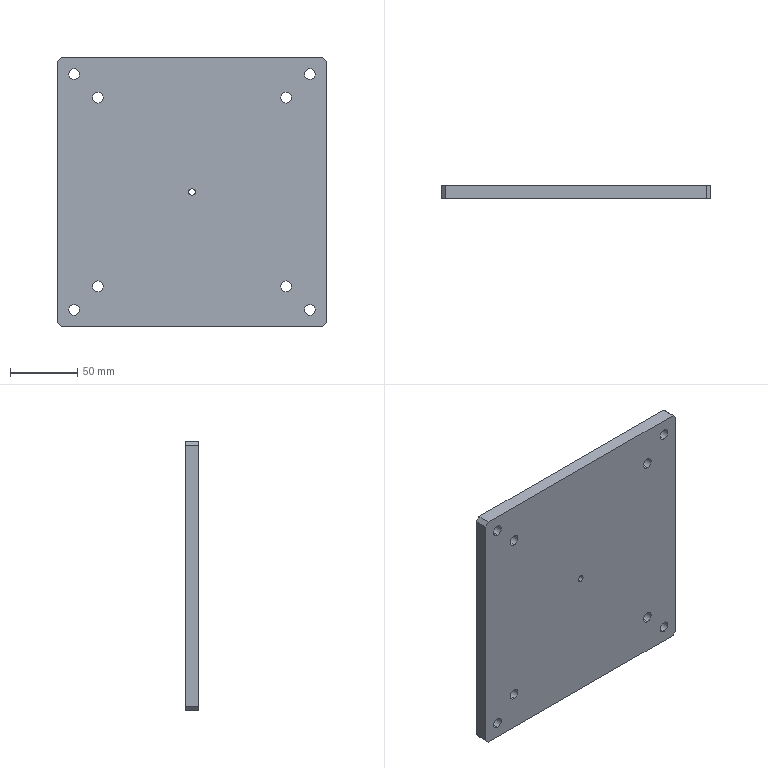Part | STEP file | Guide wheel mechanism revised.sldasm-Part-319 | 1 solid | 28 faces | box 200 x 10 x 200 mm | volume 395602 mm3 | cylinder 18 | plane 10 | commonest cylinder face diameters 8 x16 5 x2
STEP:
#1=CARTESIAN_POINT('',(-70.,10.,66.));
#2=VERTEX_POINT('',#1);
#3=CARTESIAN_POINT('',(-70.,10.,74.));
#4=VERTEX_POINT('',#3);
#5=CARTESIAN_POINT('',(-70.,10.,70.));
#6=DIRECTION('',(0.,1.,0.));
#7=DIRECTION('',(0.,0.,1.));
#8=AXIS2_PLACEMENT_3D('',#5,#6,#7);
#9=CIRCLE('',#8,4.);
#10=EDGE_CURVE('',#2,#4,#9,.T.);
#11=ORIENTED_EDGE('',*,*,#10,.T.);
#12=CARTESIAN_POINT('',(-70.,0.,74.));
#13=VERTEX_POINT('',#12);
#14=CARTESIAN_POINT('',(-70.,10.,74.));
#15=DIRECTION('',(0.,-1.,0.));
#16=VECTOR('',#15,1000.);
#17=LINE('',#14,#16);
#18=EDGE_CURVE('',#4,#13,#17,.T.);
#19=ORIENTED_EDGE('',*,*,#18,.T.);
#20=CARTESIAN_POINT('',(-70.,0.,66.));
#21=VERTEX_POINT('',#20);
#22=CARTESIAN_POINT('',(-70.,0.,70.));
#23=DIRECTION('',(0.,1.,0.));
#24=DIRECTION('',(0.,0.,1.));
#25=AXIS2_PLACEMENT_3D('',#22,#23,#24);
#26=CIRCLE('',#25,4.);
#27=EDGE_CURVE('',#21,#13,#26,.T.);
#28=ORIENTED_EDGE('',*,*,#27,.F.);
#29=CARTESIAN_POINT('',(-70.,10.,66.));
#30=DIRECTION('',(0.,-1.,0.));
#31=VECTOR('',#30,1000.);
#32=LINE('',#29,#31);
#33=EDGE_CURVE('',#2,#21,#32,.T.);
#34=ORIENTED_EDGE('',*,*,#33,.F.);
#35=EDGE_LOOP('',(#11,#19,#28,#34));
#36=FACE_OUTER_BOUND('',#35,.T.);
#37=CARTESIAN_POINT('',(-70.,10.,70.));
#38=DIRECTION('',(0.,-1.,0.));
#39=DIRECTION('',(0.,0.,-1.));
#40=AXIS2_PLACEMENT_3D('',#37,#38,#39);
#41=CYLINDRICAL_SURFACE('',#40,4.);
#42=ADVANCED_FACE('',(#36),#41,.F.);
#43=CARTESIAN_POINT('',(70.,10.,66.));
#44=VERTEX_POINT('',#43);
#45=CARTESIAN_POINT('',(70.,10.,74.));
#46=VERTEX_POINT('',#45);
#47=CARTESIAN_POINT('',(70.,10.,70.));
#48=DIRECTION('',(0.,1.,0.));
#49=DIRECTION('',(0.,0.,1.));
#50=AXIS2_PLACEMENT_3D('',#47,#48,#49);
#51=CIRCLE('',#50,4.);
#52=EDGE_CURVE('',#44,#46,#51,.T.);
#53=ORIENTED_EDGE('',*,*,#52,.T.);
#54=CARTESIAN_POINT('',(70.,0.,74.));
#55=VERTEX_POINT('',#54);
#56=CARTESIAN_POINT('',(70.,10.,74.));
#57=DIRECTION('',(0.,-1.,0.));
#58=VECTOR('',#57,1000.);
#59=LINE('',#56,#58);
#60=EDGE_CURVE('',#46,#55,#59,.T.);
#61=ORIENTED_EDGE('',*,*,#60,.T.);
#62=CARTESIAN_POINT('',(70.,0.,66.));
#63=VERTEX_POINT('',#62);
#64=CARTESIAN_POINT('',(70.,0.,70.));
#65=DIRECTION('',(0.,1.,0.));
#66=DIRECTION('',(0.,0.,1.));
#67=AXIS2_PLACEMENT_3D('',#64,#65,#66);
#68=CIRCLE('',#67,4.);
#69=EDGE_CURVE('',#63,#55,#68,.T.);
#70=ORIENTED_EDGE('',*,*,#69,.F.);
#71=CARTESIAN_POINT('',(70.,10.,66.));
#72=DIRECTION('',(0.,-1.,0.));
#73=VECTOR('',#72,1000.);
#74=LINE('',#71,#73);
#75=EDGE_CURVE('',#44,#63,#74,.T.);
#76=ORIENTED_EDGE('',*,*,#75,.F.);
#77=EDGE_LOOP('',(#53,#61,#70,#76));
#78=FACE_OUTER_BOUND('',#77,.T.);
#79=CARTESIAN_POINT('',(70.,10.,70.));
#80=DIRECTION('',(0.,-1.,0.));
#81=DIRECTION('',(0.,0.,-1.));
#82=AXIS2_PLACEMENT_3D('',#79,#80,#81);
#83=CYLINDRICAL_SURFACE('',#82,4.);
#84=ADVANCED_FACE('',(#78),#83,.F.);
#85=CARTESIAN_POINT('',(70.,10.,-74.));
#86=VERTEX_POINT('',#85);
#87=CARTESIAN_POINT('',(70.,10.,-66.));
#88=VERTEX_POINT('',#87);
#89=CARTESIAN_POINT('',(70.,10.,-70.));
#90=DIRECTION('',(0.,1.,0.));
#91=DIRECTION('',(0.,0.,1.));
#92=AXIS2_PLACEMENT_3D('',#89,#90,#91);
#93=CIRCLE('',#92,4.);
#94=EDGE_CURVE('',#86,#88,#93,.T.);
#95=ORIENTED_EDGE('',*,*,#94,.T.);
#96=CARTESIAN_POINT('',(70.,0.,-66.));
#97=VERTEX_POINT('',#96);
#98=CARTESIAN_POINT('',(70.,10.,-66.));
#99=DIRECTION('',(0.,-1.,0.));
#100=VECTOR('',#99,1000.);
#101=LINE('',#98,#100);
#102=EDGE_CURVE('',#88,#97,#101,.T.);
#103=ORIENTED_EDGE('',*,*,#102,.T.);
#104=CARTESIAN_POINT('',(70.,0.,-74.));
#105=VERTEX_POINT('',#104);
#106=CARTESIAN_POINT('',(70.,0.,-70.));
#107=DIRECTION('',(0.,1.,0.));
#108=DIRECTION('',(0.,0.,1.));
#109=AXIS2_PLACEMENT_3D('',#106,#107,#108);
#110=CIRCLE('',#109,4.);
#111=EDGE_CURVE('',#105,#97,#110,.T.);
#112=ORIENTED_EDGE('',*,*,#111,.F.);
#113=CARTESIAN_POINT('',(70.,10.,-74.));
#114=DIRECTION('',(0.,-1.,0.));
#115=VECTOR('',#114,1000.);
#116=LINE('',#113,#115);
#117=EDGE_CURVE('',#86,#105,#116,.T.);
#118=ORIENTED_EDGE('',*,*,#117,.F.);
#119=EDGE_LOOP('',(#95,#103,#112,#118));
#120=FACE_OUTER_BOUND('',#119,.T.);
#121=CARTESIAN_POINT('',(70.,10.,-70.));
#122=DIRECTION('',(0.,-1.,0.));
#123=DIRECTION('',(0.,0.,-1.));
#124=AXIS2_PLACEMENT_3D('',#121,#122,#123);
#125=CYLINDRICAL_SURFACE('',#124,4.);
#126=ADVANCED_FACE('',(#120),#125,.F.);
#127=CARTESIAN_POINT('',(-70.,10.,-74.));
#128=VERTEX_POINT('',#127);
#129=CARTESIAN_POINT('',(-70.,10.,-66.));
#130=VERTEX_POINT('',#129);
#131=CARTESIAN_POINT('',(-70.,10.,-70.));
#132=DIRECTION('',(0.,1.,0.));
#133=DIRECTION('',(0.,0.,1.));
#134=AXIS2_PLACEMENT_3D('',#131,#132,#133);
#135=CIRCLE('',#134,4.);
#136=EDGE_CURVE('',#128,#130,#135,.T.);
#137=ORIENTED_EDGE('',*,*,#136,.T.);
#138=CARTESIAN_POINT('',(-70.,0.,-66.));
#139=VERTEX_POINT('',#138);
#140=CARTESIAN_POINT('',(-70.,10.,-66.));
#141=DIRECTION('',(0.,-1.,0.));
#142=VECTOR('',#141,1000.);
#143=LINE('',#140,#142);
#144=EDGE_CURVE('',#130,#139,#143,.T.);
#145=ORIENTED_EDGE('',*,*,#144,.T.);
#146=CARTESIAN_POINT('',(-70.,0.,-74.));
#147=VERTEX_POINT('',#146);
#148=CARTESIAN_POINT('',(-70.,0.,-70.));
#149=DIRECTION('',(0.,1.,0.));
#150=DIRECTION('',(0.,0.,1.));
#151=AXIS2_PLACEMENT_3D('',#148,#149,#150);
#152=CIRCLE('',#151,4.);
#153=EDGE_CURVE('',#147,#139,#152,.T.);
#154=ORIENTED_EDGE('',*,*,#153,.F.);
#155=CARTESIAN_POINT('',(-70.,10.,-74.));
#156=DIRECTION('',(0.,-1.,0.));
#157=VECTOR('',#156,1000.);
#158=LINE('',#155,#157);
#159=EDGE_CURVE('',#128,#147,#158,.T.);
#160=ORIENTED_EDGE('',*,*,#159,.F.);
#161=EDGE_LOOP('',(#137,#145,#154,#160));
#162=FACE_OUTER_BOUND('',#161,.T.);
#163=CARTESIAN_POINT('',(-70.,10.,-70.));
#164=DIRECTION('',(0.,-1.,0.));
#165=DIRECTION('',(0.,0.,-1.));
#166=AXIS2_PLACEMENT_3D('',#163,#164,#165);
#167=CYLINDRICAL_SURFACE('',#166,4.);
#168=ADVANCED_FACE('',(#162),#167,.F.);
#169=CARTESIAN_POINT('',(-87.5,10.,83.5));
#170=VERTEX_POINT('',#169);
#171=CARTESIAN_POINT('',(-87.5,10.,91.5));
#172=VERTEX_POINT('',#171);
#173=CARTESIAN_POINT('',(-87.5,10.,87.5));
#174=DIRECTION('',(0.,1.,0.));
#175=DIRECTION('',(0.,0.,1.));
#176=AXIS2_PLACEMENT_3D('',#173,#174,#175);
#177=CIRCLE('',#176,4.);
#178=EDGE_CURVE('',#170,#172,#177,.T.);
#179=ORIENTED_EDGE('',*,*,#178,.T.);
#180=CARTESIAN_POINT('',(-87.5,0.,91.5));
#181=VERTEX_POINT('',#180);
#182=CARTESIAN_POINT('',(-87.5,10.,91.5));
#183=DIRECTION('',(0.,-1.,0.));
#184=VECTOR('',#183,1000.);
#185=LINE('',#182,#184);
#186=EDGE_CURVE('',#172,#181,#185,.T.);
#187=ORIENTED_EDGE('',*,*,#186,.T.);
#188=CARTESIAN_POINT('',(-87.5,0.,83.5));
#189=VERTEX_POINT('',#188);
#190=CARTESIAN_POINT('',(-87.5,0.,87.5));
#191=DIRECTION('',(0.,1.,0.));
#192=DIRECTION('',(0.,0.,1.));
#193=AXIS2_PLACEMENT_3D('',#190,#191,#192);
#194=CIRCLE('',#193,4.);
#195=EDGE_CURVE('',#189,#181,#194,.T.);
#196=ORIENTED_EDGE('',*,*,#195,.F.);
#197=CARTESIAN_POINT('',(-87.5,10.,83.5));
#198=DIRECTION('',(0.,-1.,0.));
#199=VECTOR('',#198,1000.);
#200=LINE('',#197,#199);
#201=EDGE_CURVE('',#170,#189,#200,.T.);
#202=ORIENTED_EDGE('',*,*,#201,.F.);
#203=EDGE_LOOP('',(#179,#187,#196,#202));
#204=FACE_OUTER_BOUND('',#203,.T.);
#205=CARTESIAN_POINT('',(-87.5,10.,87.5));
#206=DIRECTION('',(0.,-1.,0.));
#207=DIRECTION('',(0.,0.,-1.));
#208=AXIS2_PLACEMENT_3D('',#205,#206,#207);
#209=CYLINDRICAL_SURFACE('',#208,4.);
#210=ADVANCED_FACE('',(#204),#209,.F.);
#211=CARTESIAN_POINT('',(87.5,10.,83.5));
#212=VERTEX_POINT('',#211);
#213=CARTESIAN_POINT('',(87.5,10.,91.5));
#214=VERTEX_POINT('',#213);
#215=CARTESIAN_POINT('',(87.5,10.,87.5));
#216=DIRECTION('',(0.,1.,0.));
#217=DIRECTION('',(0.,0.,1.));
#218=AXIS2_PLACEMENT_3D('',#215,#216,#217);
#219=CIRCLE('',#218,4.);
#220=EDGE_CURVE('',#212,#214,#219,.T.);
#221=ORIENTED_EDGE('',*,*,#220,.T.);
#222=CARTESIAN_POINT('',(87.5,0.,91.5));
#223=VERTEX_POINT('',#222);
#224=CARTESIAN_POINT('',(87.5,10.,91.5));
#225=DIRECTION('',(0.,-1.,0.));
#226=VECTOR('',#225,1000.);
#227=LINE('',#224,#226);
#228=EDGE_CURVE('',#214,#223,#227,.T.);
#229=ORIENTED_EDGE('',*,*,#228,.T.);
#230=CARTESIAN_POINT('',(87.5,0.,83.5));
#231=VERTEX_POINT('',#230);
#232=CARTESIAN_POINT('',(87.5,0.,87.5));
#233=DIRECTION('',(0.,1.,0.));
#234=DIRECTION('',(0.,0.,1.));
#235=AXIS2_PLACEMENT_3D('',#232,#233,#234);
#236=CIRCLE('',#235,4.);
#237=EDGE_CURVE('',#231,#223,#236,.T.);
#238=ORIENTED_EDGE('',*,*,#237,.F.);
#239=CARTESIAN_POINT('',(87.5,10.,83.5));
#240=DIRECTION('',(0.,-1.,0.));
#241=VECTOR('',#240,1000.);
#242=LINE('',#239,#241);
#243=EDGE_CURVE('',#212,#231,#242,.T.);
#244=ORIENTED_EDGE('',*,*,#243,.F.);
#245=EDGE_LOOP('',(#221,#229,#238,#244));
#246=FACE_OUTER_BOUND('',#245,.T.);
#247=CARTESIAN_POINT('',(87.5,10.,87.5));
#248=DIRECTION('',(0.,-1.,0.));
#249=DIRECTION('',(0.,0.,-1.));
#250=AXIS2_PLACEMENT_3D('',#247,#248,#249);
#251=CYLINDRICAL_SURFACE('',#250,4.);
#252=ADVANCED_FACE('',(#246),#251,.F.);
#253=CARTESIAN_POINT('',(87.5,10.,-91.5));
#254=VERTEX_POINT('',#253);
#255=CARTESIAN_POINT('',(87.5,10.,-83.5));
#256=VERTEX_POINT('',#255);
#257=CARTESIAN_POINT('',(87.5,10.,-87.5));
#258=DIRECTION('',(0.,1.,0.));
#259=DIRECTION('',(0.,0.,1.));
#260=AXIS2_PLACEMENT_3D('',#257,#258,#259);
#261=CIRCLE('',#260,4.);
#262=EDGE_CURVE('',#254,#256,#261,.T.);
#263=ORIENTED_EDGE('',*,*,#262,.T.);
#264=CARTESIAN_POINT('',(87.5,0.,-83.5));
#265=VERTEX_POINT('',#264);
#266=CARTESIAN_POINT('',(87.5,10.,-83.5));
#267=DIRECTION('',(0.,-1.,0.));
#268=VECTOR('',#267,1000.);
#269=LINE('',#266,#268);
#270=EDGE_CURVE('',#256,#265,#269,.T.);
#271=ORIENTED_EDGE('',*,*,#270,.T.);
#272=CARTESIAN_POINT('',(87.5,0.,-91.5));
#273=VERTEX_POINT('',#272);
#274=CARTESIAN_POINT('',(87.5,0.,-87.5));
#275=DIRECTION('',(0.,1.,0.));
#276=DIRECTION('',(0.,0.,1.));
#277=AXIS2_PLACEMENT_3D('',#274,#275,#276);
#278=CIRCLE('',#277,4.);
#279=EDGE_CURVE('',#273,#265,#278,.T.);
#280=ORIENTED_EDGE('',*,*,#279,.F.);
#281=CARTESIAN_POINT('',(87.5,10.,-91.5));
#282=DIRECTION('',(0.,-1.,0.));
#283=VECTOR('',#282,1000.);
#284=LINE('',#281,#283);
#285=EDGE_CURVE('',#254,#273,#284,.T.);
#286=ORIENTED_EDGE('',*,*,#285,.F.);
#287=EDGE_LOOP('',(#263,#271,#280,#286));
#288=FACE_OUTER_BOUND('',#287,.T.);
#289=CARTESIAN_POINT('',(87.5,10.,-87.5));
#290=DIRECTION('',(0.,-1.,0.));
#291=DIRECTION('',(0.,0.,-1.));
#292=AXIS2_PLACEMENT_3D('',#289,#290,#291);
#293=CYLINDRICAL_SURFACE('',#292,4.);
#294=ADVANCED_FACE('',(#288),#293,.F.);
#295=CARTESIAN_POINT('',(-87.5,10.,-91.5));
#296=VERTEX_POINT('',#295);
#297=CARTESIAN_POINT('',(-87.5,10.,-83.5));
#298=VERTEX_POINT('',#297);
#299=CARTESIAN_POINT('',(-87.5,10.,-87.5));
#300=DIRECTION('',(0.,1.,0.));
#301=DIRECTION('',(0.,0.,1.));
#302=AXIS2_PLACEMENT_3D('',#299,#300,#301);
#303=CIRCLE('',#302,4.);
#304=EDGE_CURVE('',#296,#298,#303,.T.);
#305=ORIENTED_EDGE('',*,*,#304,.T.);
#306=CARTESIAN_POINT('',(-87.5,0.,-83.5));
#307=VERTEX_POINT('',#306);
#308=CARTESIAN_POINT('',(-87.5,10.,-83.5));
#309=DIRECTION('',(0.,-1.,0.));
#310=VECTOR('',#309,1000.);
#311=LINE('',#308,#310);
#312=EDGE_CURVE('',#298,#307,#311,.T.);
#313=ORIENTED_EDGE('',*,*,#312,.T.);
#314=CARTESIAN_POINT('',(-87.5,0.,-91.5));
#315=VERTEX_POINT('',#314);
#316=CARTESIAN_POINT('',(-87.5,0.,-87.5));
#317=DIRECTION('',(0.,1.,0.));
#318=DIRECTION('',(0.,0.,1.));
#319=AXIS2_PLACEMENT_3D('',#316,#317,#318);
#320=CIRCLE('',#319,4.);
#321=EDGE_CURVE('',#315,#307,#320,.T.);
#322=ORIENTED_EDGE('',*,*,#321,.F.);
#323=CARTESIAN_POINT('',(-87.5,10.,-91.5));
#324=DIRECTION('',(0.,-1.,0.));
#325=VECTOR('',#324,1000.);
#326=LINE('',#323,#325);
#327=EDGE_CURVE('',#296,#315,#326,.T.);
#328=ORIENTED_EDGE('',*,*,#327,.F.);
#329=EDGE_LOOP('',(#305,#313,#322,#328));
#330=FACE_OUTER_BOUND('',#329,.T.);
#331=CARTESIAN_POINT('',(-87.5,10.,-87.5));
#332=DIRECTION('',(0.,-1.,0.));
#333=DIRECTION('',(0.,0.,-1.));
#334=AXIS2_PLACEMENT_3D('',#331,#332,#333);
#335=CYLINDRICAL_SURFACE('',#334,4.);
#336=ADVANCED_FACE('',(#330),#335,.F.);
#337=CARTESIAN_POINT('',(0.,10.,-2.5));
#338=VERTEX_POINT('',#337);
#339=CARTESIAN_POINT('',(0.,10.,2.5));
#340=VERTEX_POINT('',#339);
#341=CARTESIAN_POINT('',(0.,10.,0.));
#342=DIRECTION('',(0.,1.,0.));
#343=DIRECTION('',(0.,0.,1.));
#344=AXIS2_PLACEMENT_3D('',#341,#342,#343);
#345=CIRCLE('',#344,2.5);
#346=EDGE_CURVE('',#338,#340,#345,.T.);
#347=ORIENTED_EDGE('',*,*,#346,.T.);
#348=CARTESIAN_POINT('',(0.,0.,2.5));
#349=VERTEX_POINT('',#348);
#350=CARTESIAN_POINT('',(0.,10.,2.5));
#351=DIRECTION('',(0.,-1.,0.));
#352=VECTOR('',#351,1000.);
#353=LINE('',#350,#352);
#354=EDGE_CURVE('',#340,#349,#353,.T.);
#355=ORIENTED_EDGE('',*,*,#354,.T.);
#356=CARTESIAN_POINT('',(0.,0.,-2.5));
#357=VERTEX_POINT('',#356);
#358=CARTESIAN_POINT('',(0.,0.,0.));
#359=DIRECTION('',(0.,1.,0.));
#360=DIRECTION('',(0.,0.,1.));
#361=AXIS2_PLACEMENT_3D('',#358,#359,#360);
#362=CIRCLE('',#361,2.5);
#363=EDGE_CURVE('',#357,#349,#362,.T.);
#364=ORIENTED_EDGE('',*,*,#363,.F.);
#365=CARTESIAN_POINT('',(0.,10.,-2.5));
#366=DIRECTION('',(0.,-1.,0.));
#367=VECTOR('',#366,1000.);
#368=LINE('',#365,#367);
#369=EDGE_CURVE('',#338,#357,#368,.T.);
#370=ORIENTED_EDGE('',*,*,#369,.F.);
#371=EDGE_LOOP('',(#347,#355,#364,#370));
#372=FACE_OUTER_BOUND('',#371,.T.);
#373=CARTESIAN_POINT('',(0.,10.,0.));
#374=DIRECTION('',(0.,-1.,0.));
#375=DIRECTION('',(0.,0.,-1.));
#376=AXIS2_PLACEMENT_3D('',#373,#374,#375);
#377=CYLINDRICAL_SURFACE('',#376,2.5);
#378=ADVANCED_FACE('',(#372),#377,.F.);
#379=ORIENTED_EDGE('',*,*,#52,.F.);
#380=CARTESIAN_POINT('',(70.,10.,70.));
#381=DIRECTION('',(0.,1.,0.));
#382=DIRECTION('',(0.,0.,1.));
#383=AXIS2_PLACEMENT_3D('',#380,#381,#382);
#384=CIRCLE('',#383,4.);
#385=EDGE_CURVE('',#46,#44,#384,.T.);
#386=ORIENTED_EDGE('',*,*,#385,.F.);
#387=EDGE_LOOP('',(#379,#386));
#388=FACE_BOUND('',#387,.T.);
#389=ORIENTED_EDGE('',*,*,#136,.F.);
#390=CARTESIAN_POINT('',(-70.,10.,-70.));
#391=DIRECTION('',(0.,1.,0.));
#392=DIRECTION('',(0.,0.,1.));
#393=AXIS2_PLACEMENT_3D('',#390,#391,#392);
#394=CIRCLE('',#393,4.);
#395=EDGE_CURVE('',#130,#128,#394,.T.);
#396=ORIENTED_EDGE('',*,*,#395,.F.);
#397=EDGE_LOOP('',(#389,#396));
#398=FACE_BOUND('',#397,.T.);
#399=ORIENTED_EDGE('',*,*,#220,.F.);
#400=CARTESIAN_POINT('',(87.5,10.,87.5));
#401=DIRECTION('',(0.,1.,0.));
#402=DIRECTION('',(0.,0.,1.));
#403=AXIS2_PLACEMENT_3D('',#400,#401,#402);
#404=CIRCLE('',#403,4.);
#405=EDGE_CURVE('',#214,#212,#404,.T.);
#406=ORIENTED_EDGE('',*,*,#405,.F.);
#407=EDGE_LOOP('',(#399,#406));
#408=FACE_BOUND('',#407,.T.);
#409=ORIENTED_EDGE('',*,*,#304,.F.);
#410=CARTESIAN_POINT('',(-87.5,10.,-87.5));
#411=DIRECTION('',(0.,1.,0.));
#412=DIRECTION('',(0.,0.,1.));
#413=AXIS2_PLACEMENT_3D('',#410,#411,#412);
#414=CIRCLE('',#413,4.);
#415=EDGE_CURVE('',#298,#296,#414,.T.);
#416=ORIENTED_EDGE('',*,*,#415,.F.);
#417=EDGE_LOOP('',(#409,#416));
#418=FACE_BOUND('',#417,.T.);
#419=CARTESIAN_POINT('',(-100.,10.,-97.));
#420=VERTEX_POINT('',#419);
#421=CARTESIAN_POINT('',(-100.,10.,97.));
#422=VERTEX_POINT('',#421);
#423=CARTESIAN_POINT('',(-100.,10.,100.));
#424=DIRECTION('',(0.,0.,1.));
#425=VECTOR('',#424,1000.);
#426=LINE('',#423,#425);
#427=EDGE_CURVE('',#420,#422,#426,.T.);
#428=ORIENTED_EDGE('',*,*,#427,.T.);
#429=CARTESIAN_POINT('',(-97.,10.,100.));
#430=VERTEX_POINT('',#429);
#431=CARTESIAN_POINT('',(-98.5,10.,98.5));
#432=DIRECTION('',(0.7071,0.,0.7071));
#433=VECTOR('',#432,1000.);
#434=LINE('',#431,#433);
#435=EDGE_CURVE('',#422,#430,#434,.T.);
#436=ORIENTED_EDGE('',*,*,#435,.T.);
#437=CARTESIAN_POINT('',(97.,10.,100.));
#438=VERTEX_POINT('',#437);
#439=CARTESIAN_POINT('',(100.,10.,100.));
#440=DIRECTION('',(1.,0.,0.));
#441=VECTOR('',#440,1000.);
#442=LINE('',#439,#441);
#443=EDGE_CURVE('',#430,#438,#442,.T.);
#444=ORIENTED_EDGE('',*,*,#443,.T.);
#445=CARTESIAN_POINT('',(100.,10.,97.));
#446=VERTEX_POINT('',#445);
#447=CARTESIAN_POINT('',(98.5,10.,98.5));
#448=DIRECTION('',(0.7071,0.,-0.7071));
#449=VECTOR('',#448,1000.);
#450=LINE('',#447,#449);
#451=EDGE_CURVE('',#438,#446,#450,.T.);
#452=ORIENTED_EDGE('',*,*,#451,.T.);
#453=CARTESIAN_POINT('',(100.,10.,-97.));
#454=VERTEX_POINT('',#453);
#455=CARTESIAN_POINT('',(100.,10.,100.));
#456=DIRECTION('',(0.,0.,-1.));
#457=VECTOR('',#456,1000.);
#458=LINE('',#455,#457);
#459=EDGE_CURVE('',#446,#454,#458,.T.);
#460=ORIENTED_EDGE('',*,*,#459,.T.);
#461=CARTESIAN_POINT('',(97.,10.,-100.));
#462=VERTEX_POINT('',#461);
#463=CARTESIAN_POINT('',(98.5,10.,-98.5));
#464=DIRECTION('',(-0.7071,0.,-0.7071));
#465=VECTOR('',#464,1000.);
#466=LINE('',#463,#465);
#467=EDGE_CURVE('',#454,#462,#466,.T.);
#468=ORIENTED_EDGE('',*,*,#467,.T.);
#469=CARTESIAN_POINT('',(-97.,10.,-100.));
#470=VERTEX_POINT('',#469);
#471=CARTESIAN_POINT('',(100.,10.,-100.));
#472=DIRECTION('',(-1.,0.,0.));
#473=VECTOR('',#472,1000.);
#474=LINE('',#471,#473);
#475=EDGE_CURVE('',#462,#470,#474,.T.);
#476=ORIENTED_EDGE('',*,*,#475,.T.);
#477=CARTESIAN_POINT('',(-98.5,10.,-98.5));
#478=DIRECTION('',(-0.7071,0.,0.7071));
#479=VECTOR('',#478,1000.);
#480=LINE('',#477,#479);
#481=EDGE_CURVE('',#470,#420,#480,.T.);
#482=ORIENTED_EDGE('',*,*,#481,.T.);
#483=EDGE_LOOP('',(#428,#436,#444,#452,#460,#468,#476,#482));
#484=FACE_OUTER_BOUND('',#483,.T.);
#485=ORIENTED_EDGE('',*,*,#346,.F.);
#486=CARTESIAN_POINT('',(0.,10.,0.));
#487=DIRECTION('',(0.,1.,0.));
#488=DIRECTION('',(0.,0.,1.));
#489=AXIS2_PLACEMENT_3D('',#486,#487,#488);
#490=CIRCLE('',#489,2.5);
#491=EDGE_CURVE('',#340,#338,#490,.T.);
#492=ORIENTED_EDGE('',*,*,#491,.F.);
#493=EDGE_LOOP('',(#485,#492));
#494=FACE_BOUND('',#493,.T.);
#495=ORIENTED_EDGE('',*,*,#262,.F.);
#496=CARTESIAN_POINT('',(87.5,10.,-87.5));
#497=DIRECTION('',(0.,1.,0.));
#498=DIRECTION('',(0.,0.,1.));
#499=AXIS2_PLACEMENT_3D('',#496,#497,#498);
#500=CIRCLE('',#499,4.);
#501=EDGE_CURVE('',#256,#254,#500,.T.);
#502=ORIENTED_EDGE('',*,*,#501,.F.);
#503=EDGE_LOOP('',(#495,#502));
#504=FACE_BOUND('',#503,.T.);
#505=ORIENTED_EDGE('',*,*,#178,.F.);
#506=CARTESIAN_POINT('',(-87.5,10.,87.5));
#507=DIRECTION('',(0.,1.,0.));
#508=DIRECTION('',(0.,0.,1.));
#509=AXIS2_PLACEMENT_3D('',#506,#507,#508);
#510=CIRCLE('',#509,4.);
#511=EDGE_CURVE('',#172,#170,#510,.T.);
#512=ORIENTED_EDGE('',*,*,#511,.F.);
#513=EDGE_LOOP('',(#505,#512));
#514=FACE_BOUND('',#513,.T.);
#515=ORIENTED_EDGE('',*,*,#94,.F.);
#516=CARTESIAN_POINT('',(70.,10.,-70.));
#517=DIRECTION('',(0.,1.,0.));
#518=DIRECTION('',(0.,0.,1.));
#519=AXIS2_PLACEMENT_3D('',#516,#517,#518);
#520=CIRCLE('',#519,4.);
#521=EDGE_CURVE('',#88,#86,#520,.T.);
#522=ORIENTED_EDGE('',*,*,#521,.F.);
#523=EDGE_LOOP('',(#515,#522));
#524=FACE_BOUND('',#523,.T.);
#525=ORIENTED_EDGE('',*,*,#10,.F.);
#526=CARTESIAN_POINT('',(-70.,10.,70.));
#527=DIRECTION('',(0.,1.,0.));
#528=DIRECTION('',(0.,0.,1.));
#529=AXIS2_PLACEMENT_3D('',#526,#527,#528);
#530=CIRCLE('',#529,4.);
#531=EDGE_CURVE('',#4,#2,#530,.T.);
#532=ORIENTED_EDGE('',*,*,#531,.F.);
#533=EDGE_LOOP('',(#525,#532));
#534=FACE_BOUND('',#533,.T.);
#535=CARTESIAN_POINT('',(0.,10.,0.));
#536=DIRECTION('',(0.,1.,0.));
#537=DIRECTION('',(0.,0.,1.));
#538=AXIS2_PLACEMENT_3D('',#535,#536,#537);
#539=PLANE('',#538);
#540=ADVANCED_FACE('',(#388,#398,#408,#418,#484,#494,#504,#514,#524,#534),#539,.T.);
#541=ORIENTED_EDGE('',*,*,#69,.T.);
#542=CARTESIAN_POINT('',(70.,0.,70.));
#543=DIRECTION('',(0.,1.,0.));
#544=DIRECTION('',(0.,0.,1.));
#545=AXIS2_PLACEMENT_3D('',#542,#543,#544);
#546=CIRCLE('',#545,4.);
#547=EDGE_CURVE('',#55,#63,#546,.T.);
#548=ORIENTED_EDGE('',*,*,#547,.T.);
#549=EDGE_LOOP('',(#541,#548));
#550=FACE_BOUND('',#549,.T.);
#551=ORIENTED_EDGE('',*,*,#153,.T.);
#552=CARTESIAN_POINT('',(-70.,0.,-70.));
#553=DIRECTION('',(0.,1.,0.));
#554=DIRECTION('',(0.,0.,1.));
#555=AXIS2_PLACEMENT_3D('',#552,#553,#554);
#556=CIRCLE('',#555,4.);
#557=EDGE_CURVE('',#139,#147,#556,.T.);
#558=ORIENTED_EDGE('',*,*,#557,.T.);
#559=EDGE_LOOP('',(#551,#558));
#560=FACE_BOUND('',#559,.T.);
#561=ORIENTED_EDGE('',*,*,#237,.T.);
#562=CARTESIAN_POINT('',(87.5,0.,87.5));
#563=DIRECTION('',(0.,1.,0.));
#564=DIRECTION('',(0.,0.,1.));
#565=AXIS2_PLACEMENT_3D('',#562,#563,#564);
#566=CIRCLE('',#565,4.);
#567=EDGE_CURVE('',#223,#231,#566,.T.);
#568=ORIENTED_EDGE('',*,*,#567,.T.);
#569=EDGE_LOOP('',(#561,#568));
#570=FACE_BOUND('',#569,.T.);
#571=ORIENTED_EDGE('',*,*,#321,.T.);
#572=CARTESIAN_POINT('',(-87.5,0.,-87.5));
#573=DIRECTION('',(0.,1.,0.));
#574=DIRECTION('',(0.,0.,1.));
#575=AXIS2_PLACEMENT_3D('',#572,#573,#574);
#576=CIRCLE('',#575,4.);
#577=EDGE_CURVE('',#307,#315,#576,.T.);
#578=ORIENTED_EDGE('',*,*,#577,.T.);
#579=EDGE_LOOP('',(#571,#578));
#580=FACE_BOUND('',#579,.T.);
#581=CARTESIAN_POINT('',(-97.,0.,100.));
#582=VERTEX_POINT('',#581);
#583=CARTESIAN_POINT('',(97.,0.,100.));
#584=VERTEX_POINT('',#583);
#585=CARTESIAN_POINT('',(100.,0.,100.));
#586=DIRECTION('',(1.,0.,0.));
#587=VECTOR('',#586,1000.);
#588=LINE('',#585,#587);
#589=EDGE_CURVE('',#582,#584,#588,.T.);
#590=ORIENTED_EDGE('',*,*,#589,.F.);
#591=CARTESIAN_POINT('',(-100.,0.,97.));
#592=VERTEX_POINT('',#591);
#593=CARTESIAN_POINT('',(-97.,0.,100.));
#594=DIRECTION('',(-0.7071,0.,-0.7071));
#595=VECTOR('',#594,1000.);
#596=LINE('',#593,#595);
#597=EDGE_CURVE('',#582,#592,#596,.T.);
#598=ORIENTED_EDGE('',*,*,#597,.T.);
#599=CARTESIAN_POINT('',(-100.,0.,-97.));
#600=VERTEX_POINT('',#599);
#601=CARTESIAN_POINT('',(-100.,0.,100.));
#602=DIRECTION('',(0.,0.,1.));
#603=VECTOR('',#602,1000.);
#604=LINE('',#601,#603);
#605=EDGE_CURVE('',#600,#592,#604,.T.);
#606=ORIENTED_EDGE('',*,*,#605,.F.);
#607=CARTESIAN_POINT('',(-97.,0.,-100.));
#608=VERTEX_POINT('',#607);
#609=CARTESIAN_POINT('',(-100.,0.,-97.));
#610=DIRECTION('',(0.7071,0.,-0.7071));
#611=VECTOR('',#610,1000.);
#612=LINE('',#609,#611);
#613=EDGE_CURVE('',#600,#608,#612,.T.);
#614=ORIENTED_EDGE('',*,*,#613,.T.);
#615=CARTESIAN_POINT('',(97.,0.,-100.));
#616=VERTEX_POINT('',#615);
#617=CARTESIAN_POINT('',(100.,0.,-100.));
#618=DIRECTION('',(-1.,0.,0.));
#619=VECTOR('',#618,1000.);
#620=LINE('',#617,#619);
#621=EDGE_CURVE('',#616,#608,#620,.T.);
#622=ORIENTED_EDGE('',*,*,#621,.F.);
#623=CARTESIAN_POINT('',(100.,0.,-97.));
#624=VERTEX_POINT('',#623);
#625=CARTESIAN_POINT('',(97.,0.,-100.));
#626=DIRECTION('',(0.7071,0.,0.7071));
#627=VECTOR('',#626,1000.);
#628=LINE('',#625,#627);
#629=EDGE_CURVE('',#616,#624,#628,.T.);
#630=ORIENTED_EDGE('',*,*,#629,.T.);
#631=CARTESIAN_POINT('',(100.,0.,97.));
#632=VERTEX_POINT('',#631);
#633=CARTESIAN_POINT('',(100.,0.,100.));
#634=DIRECTION('',(0.,0.,-1.));
#635=VECTOR('',#634,1000.);
#636=LINE('',#633,#635);
#637=EDGE_CURVE('',#632,#624,#636,.T.);
#638=ORIENTED_EDGE('',*,*,#637,.F.);
#639=CARTESIAN_POINT('',(100.,0.,97.));
#640=DIRECTION('',(-0.7071,0.,0.7071));
#641=VECTOR('',#640,1000.);
#642=LINE('',#639,#641);
#643=EDGE_CURVE('',#632,#584,#642,.T.);
#644=ORIENTED_EDGE('',*,*,#643,.T.);
#645=EDGE_LOOP('',(#590,#598,#606,#614,#622,#630,#638,#644));
#646=FACE_OUTER_BOUND('',#645,.T.);
#647=ORIENTED_EDGE('',*,*,#363,.T.);
#648=CARTESIAN_POINT('',(0.,0.,0.));
#649=DIRECTION('',(0.,1.,0.));
#650=DIRECTION('',(0.,0.,1.));
#651=AXIS2_PLACEMENT_3D('',#648,#649,#650);
#652=CIRCLE('',#651,2.5);
#653=EDGE_CURVE('',#349,#357,#652,.T.);
#654=ORIENTED_EDGE('',*,*,#653,.T.);
#655=EDGE_LOOP('',(#647,#654));
#656=FACE_BOUND('',#655,.T.);
#657=ORIENTED_EDGE('',*,*,#279,.T.);
#658=CARTESIAN_POINT('',(87.5,0.,-87.5));
#659=DIRECTION('',(0.,1.,0.));
#660=DIRECTION('',(0.,0.,1.));
#661=AXIS2_PLACEMENT_3D('',#658,#659,#660);
#662=CIRCLE('',#661,4.);
#663=EDGE_CURVE('',#265,#273,#662,.T.);
#664=ORIENTED_EDGE('',*,*,#663,.T.);
#665=EDGE_LOOP('',(#657,#664));
#666=FACE_BOUND('',#665,.T.);
#667=ORIENTED_EDGE('',*,*,#195,.T.);
#668=CARTESIAN_POINT('',(-87.5,0.,87.5));
#669=DIRECTION('',(0.,1.,0.));
#670=DIRECTION('',(0.,0.,1.));
#671=AXIS2_PLACEMENT_3D('',#668,#669,#670);
#672=CIRCLE('',#671,4.);
#673=EDGE_CURVE('',#181,#189,#672,.T.);
#674=ORIENTED_EDGE('',*,*,#673,.T.);
#675=EDGE_LOOP('',(#667,#674));
#676=FACE_BOUND('',#675,.T.);
#677=ORIENTED_EDGE('',*,*,#111,.T.);
#678=CARTESIAN_POINT('',(70.,0.,-70.));
#679=DIRECTION('',(0.,1.,0.));
#680=DIRECTION('',(0.,0.,1.));
#681=AXIS2_PLACEMENT_3D('',#678,#679,#680);
#682=CIRCLE('',#681,4.);
#683=EDGE_CURVE('',#97,#105,#682,.T.);
#684=ORIENTED_EDGE('',*,*,#683,.T.);
#685=EDGE_LOOP('',(#677,#684));
#686=FACE_BOUND('',#685,.T.);
#687=ORIENTED_EDGE('',*,*,#27,.T.);
#688=CARTESIAN_POINT('',(-70.,0.,70.));
#689=DIRECTION('',(0.,1.,0.));
#690=DIRECTION('',(0.,0.,1.));
#691=AXIS2_PLACEMENT_3D('',#688,#689,#690);
#692=CIRCLE('',#691,4.);
#693=EDGE_CURVE('',#13,#21,#692,.T.);
#694=ORIENTED_EDGE('',*,*,#693,.T.);
#695=EDGE_LOOP('',(#687,#694));
#696=FACE_BOUND('',#695,.T.);
#697=CARTESIAN_POINT('',(0.,0.,0.));
#698=DIRECTION('',(0.,1.,0.));
#699=DIRECTION('',(0.,0.,1.));
#700=AXIS2_PLACEMENT_3D('',#697,#698,#699);
#701=PLANE('',#700);
#702=ADVANCED_FACE('',(#550,#560,#570,#580,#646,#656,#666,#676,#686,#696),#701,.F.);
#703=ORIENTED_EDGE('',*,*,#605,.T.);
#704=CARTESIAN_POINT('',(-100.,10.,97.));
#705=DIRECTION('',(0.,1.,0.));
#706=VECTOR('',#705,1000.);
#707=LINE('',#704,#706);
#708=EDGE_CURVE('',#592,#422,#707,.T.);
#709=ORIENTED_EDGE('',*,*,#708,.T.);
#710=ORIENTED_EDGE('',*,*,#427,.F.);
#711=CARTESIAN_POINT('',(-100.,10.,-97.));
#712=DIRECTION('',(0.,-1.,0.));
#713=VECTOR('',#712,1000.);
#714=LINE('',#711,#713);
#715=EDGE_CURVE('',#420,#600,#714,.T.);
#716=ORIENTED_EDGE('',*,*,#715,.T.);
#717=EDGE_LOOP('',(#703,#709,#710,#716));
#718=FACE_OUTER_BOUND('',#717,.T.);
#719=CARTESIAN_POINT('',(-100.,10.,100.));
#720=DIRECTION('',(1.,0.,0.));
#721=DIRECTION('',(0.,0.,-1.));
#722=AXIS2_PLACEMENT_3D('',#719,#720,#721);
#723=PLANE('',#722);
#724=ADVANCED_FACE('',(#718),#723,.F.);
#725=ORIENTED_EDGE('',*,*,#443,.F.);
#726=CARTESIAN_POINT('',(-97.,10.,100.));
#727=DIRECTION('',(0.,-1.,0.));
#728=VECTOR('',#727,1000.);
#729=LINE('',#726,#728);
#730=EDGE_CURVE('',#430,#582,#729,.T.);
#731=ORIENTED_EDGE('',*,*,#730,.T.);
#732=ORIENTED_EDGE('',*,*,#589,.T.);
#733=CARTESIAN_POINT('',(97.,10.,100.));
#734=DIRECTION('',(0.,1.,0.));
#735=VECTOR('',#734,1000.);
#736=LINE('',#733,#735);
#737=EDGE_CURVE('',#584,#438,#736,.T.);
#738=ORIENTED_EDGE('',*,*,#737,.T.);
#739=EDGE_LOOP('',(#725,#731,#732,#738));
#740=FACE_OUTER_BOUND('',#739,.T.);
#741=CARTESIAN_POINT('',(100.,10.,100.));
#742=DIRECTION('',(0.,0.,-1.));
#743=DIRECTION('',(-1.,0.,0.));
#744=AXIS2_PLACEMENT_3D('',#741,#742,#743);
#745=PLANE('',#744);
#746=ADVANCED_FACE('',(#740),#745,.F.);
#747=ORIENTED_EDGE('',*,*,#459,.F.);
#748=CARTESIAN_POINT('',(100.,10.,97.));
#749=DIRECTION('',(0.,-1.,0.));
#750=VECTOR('',#749,1000.);
#751=LINE('',#748,#750);
#752=EDGE_CURVE('',#446,#632,#751,.T.);
#753=ORIENTED_EDGE('',*,*,#752,.T.);
#754=ORIENTED_EDGE('',*,*,#637,.T.);
#755=CARTESIAN_POINT('',(100.,10.,-97.));
#756=DIRECTION('',(0.,1.,0.));
#757=VECTOR('',#756,1000.);
#758=LINE('',#755,#757);
#759=EDGE_CURVE('',#624,#454,#758,.T.);
#760=ORIENTED_EDGE('',*,*,#759,.T.);
#761=EDGE_LOOP('',(#747,#753,#754,#760));
#762=FACE_OUTER_BOUND('',#761,.T.);
#763=CARTESIAN_POINT('',(100.,10.,100.));
#764=DIRECTION('',(-1.,0.,0.));
#765=DIRECTION('',(0.,0.,1.));
#766=AXIS2_PLACEMENT_3D('',#763,#764,#765);
#767=PLANE('',#766);
#768=ADVANCED_FACE('',(#762),#767,.F.);
#769=ORIENTED_EDGE('',*,*,#475,.F.);
#770=CARTESIAN_POINT('',(97.,10.,-100.));
#771=DIRECTION('',(0.,-1.,0.));
#772=VECTOR('',#771,1000.);
#773=LINE('',#770,#772);
#774=EDGE_CURVE('',#462,#616,#773,.T.);
#775=ORIENTED_EDGE('',*,*,#774,.T.);
#776=ORIENTED_EDGE('',*,*,#621,.T.);
#777=CARTESIAN_POINT('',(-97.,10.,-100.));
#778=DIRECTION('',(0.,1.,0.));
#779=VECTOR('',#778,1000.);
#780=LINE('',#777,#779);
#781=EDGE_CURVE('',#608,#470,#780,.T.);
#782=ORIENTED_EDGE('',*,*,#781,.T.);
#783=EDGE_LOOP('',(#769,#775,#776,#782));
#784=FACE_OUTER_BOUND('',#783,.T.);
#785=CARTESIAN_POINT('',(100.,10.,-100.));
#786=DIRECTION('',(0.,0.,1.));
#787=DIRECTION('',(1.,0.,0.));
#788=AXIS2_PLACEMENT_3D('',#785,#786,#787);
#789=PLANE('',#788);
#790=ADVANCED_FACE('',(#784),#789,.F.);
#791=ORIENTED_EDGE('',*,*,#354,.F.);
#792=ORIENTED_EDGE('',*,*,#491,.T.);
#793=ORIENTED_EDGE('',*,*,#369,.T.);
#794=ORIENTED_EDGE('',*,*,#653,.F.);
#795=EDGE_LOOP('',(#791,#792,#793,#794));
#796=FACE_OUTER_BOUND('',#795,.T.);
#797=CARTESIAN_POINT('',(0.,10.,0.));
#798=DIRECTION('',(0.,-1.,0.));
#799=DIRECTION('',(0.,0.,-1.));
#800=AXIS2_PLACEMENT_3D('',#797,#798,#799);
#801=CYLINDRICAL_SURFACE('',#800,2.5);
#802=ADVANCED_FACE('',(#796),#801,.F.);
#803=ORIENTED_EDGE('',*,*,#312,.F.);
#804=ORIENTED_EDGE('',*,*,#415,.T.);
#805=ORIENTED_EDGE('',*,*,#327,.T.);
#806=ORIENTED_EDGE('',*,*,#577,.F.);
#807=EDGE_LOOP('',(#803,#804,#805,#806));
#808=FACE_OUTER_BOUND('',#807,.T.);
#809=CARTESIAN_POINT('',(-87.5,10.,-87.5));
#810=DIRECTION('',(0.,-1.,0.));
#811=DIRECTION('',(0.,0.,-1.));
#812=AXIS2_PLACEMENT_3D('',#809,#810,#811);
#813=CYLINDRICAL_SURFACE('',#812,4.);
#814=ADVANCED_FACE('',(#808),#813,.F.);
#815=ORIENTED_EDGE('',*,*,#270,.F.);
#816=ORIENTED_EDGE('',*,*,#501,.T.);
#817=ORIENTED_EDGE('',*,*,#285,.T.);
#818=ORIENTED_EDGE('',*,*,#663,.F.);
#819=EDGE_LOOP('',(#815,#816,#817,#818));
#820=FACE_OUTER_BOUND('',#819,.T.);
#821=CARTESIAN_POINT('',(87.5,10.,-87.5));
#822=DIRECTION('',(0.,-1.,0.));
#823=DIRECTION('',(0.,0.,-1.));
#824=AXIS2_PLACEMENT_3D('',#821,#822,#823);
#825=CYLINDRICAL_SURFACE('',#824,4.);
#826=ADVANCED_FACE('',(#820),#825,.F.);
#827=ORIENTED_EDGE('',*,*,#228,.F.);
#828=ORIENTED_EDGE('',*,*,#405,.T.);
#829=ORIENTED_EDGE('',*,*,#243,.T.);
#830=ORIENTED_EDGE('',*,*,#567,.F.);
#831=EDGE_LOOP('',(#827,#828,#829,#830));
#832=FACE_OUTER_BOUND('',#831,.T.);
#833=CARTESIAN_POINT('',(87.5,10.,87.5));
#834=DIRECTION('',(0.,-1.,0.));
#835=DIRECTION('',(0.,0.,-1.));
#836=AXIS2_PLACEMENT_3D('',#833,#834,#835);
#837=CYLINDRICAL_SURFACE('',#836,4.);
#838=ADVANCED_FACE('',(#832),#837,.F.);
#839=ORIENTED_EDGE('',*,*,#186,.F.);
#840=ORIENTED_EDGE('',*,*,#511,.T.);
#841=ORIENTED_EDGE('',*,*,#201,.T.);
#842=ORIENTED_EDGE('',*,*,#673,.F.);
#843=EDGE_LOOP('',(#839,#840,#841,#842));
#844=FACE_OUTER_BOUND('',#843,.T.);
#845=CARTESIAN_POINT('',(-87.5,10.,87.5));
#846=DIRECTION('',(0.,-1.,0.));
#847=DIRECTION('',(0.,0.,-1.));
#848=AXIS2_PLACEMENT_3D('',#845,#846,#847);
#849=CYLINDRICAL_SURFACE('',#848,4.);
#850=ADVANCED_FACE('',(#844),#849,.F.);
#851=ORIENTED_EDGE('',*,*,#144,.F.);
#852=ORIENTED_EDGE('',*,*,#395,.T.);
#853=ORIENTED_EDGE('',*,*,#159,.T.);
#854=ORIENTED_EDGE('',*,*,#557,.F.);
#855=EDGE_LOOP('',(#851,#852,#853,#854));
#856=FACE_OUTER_BOUND('',#855,.T.);
#857=CARTESIAN_POINT('',(-70.,10.,-70.));
#858=DIRECTION('',(0.,-1.,0.));
#859=DIRECTION('',(0.,0.,-1.));
#860=AXIS2_PLACEMENT_3D('',#857,#858,#859);
#861=CYLINDRICAL_SURFACE('',#860,4.);
#862=ADVANCED_FACE('',(#856),#861,.F.);
#863=ORIENTED_EDGE('',*,*,#102,.F.);
#864=ORIENTED_EDGE('',*,*,#521,.T.);
#865=ORIENTED_EDGE('',*,*,#117,.T.);
#866=ORIENTED_EDGE('',*,*,#683,.F.);
#867=EDGE_LOOP('',(#863,#864,#865,#866));
#868=FACE_OUTER_BOUND('',#867,.T.);
#869=CARTESIAN_POINT('',(70.,10.,-70.));
#870=DIRECTION('',(0.,-1.,0.));
#871=DIRECTION('',(0.,0.,-1.));
#872=AXIS2_PLACEMENT_3D('',#869,#870,#871);
#873=CYLINDRICAL_SURFACE('',#872,4.);
#874=ADVANCED_FACE('',(#868),#873,.F.);
#875=ORIENTED_EDGE('',*,*,#60,.F.);
#876=ORIENTED_EDGE('',*,*,#385,.T.);
#877=ORIENTED_EDGE('',*,*,#75,.T.);
#878=ORIENTED_EDGE('',*,*,#547,.F.);
#879=EDGE_LOOP('',(#875,#876,#877,#878));
#880=FACE_OUTER_BOUND('',#879,.T.);
#881=CARTESIAN_POINT('',(70.,10.,70.));
#882=DIRECTION('',(0.,-1.,0.));
#883=DIRECTION('',(0.,0.,-1.));
#884=AXIS2_PLACEMENT_3D('',#881,#882,#883);
#885=CYLINDRICAL_SURFACE('',#884,4.);
#886=ADVANCED_FACE('',(#880),#885,.F.);
#887=ORIENTED_EDGE('',*,*,#18,.F.);
#888=ORIENTED_EDGE('',*,*,#531,.T.);
#889=ORIENTED_EDGE('',*,*,#33,.T.);
#890=ORIENTED_EDGE('',*,*,#693,.F.);
#891=EDGE_LOOP('',(#887,#888,#889,#890));
#892=FACE_OUTER_BOUND('',#891,.T.);
#893=CARTESIAN_POINT('',(-70.,10.,70.));
#894=DIRECTION('',(0.,-1.,0.));
#895=DIRECTION('',(0.,0.,-1.));
#896=AXIS2_PLACEMENT_3D('',#893,#894,#895);
#897=CYLINDRICAL_SURFACE('',#896,4.);
#898=ADVANCED_FACE('',(#892),#897,.F.);
#899=ORIENTED_EDGE('',*,*,#435,.F.);
#900=ORIENTED_EDGE('',*,*,#708,.F.);
#901=ORIENTED_EDGE('',*,*,#597,.F.);
#902=ORIENTED_EDGE('',*,*,#730,.F.);
#903=EDGE_LOOP('',(#899,#900,#901,#902));
#904=FACE_OUTER_BOUND('',#903,.T.);
#905=CARTESIAN_POINT('',(-97.,10.,100.));
#906=DIRECTION('',(0.7071,0.,-0.7071));
#907=DIRECTION('',(0.,-1.,0.));
#908=AXIS2_PLACEMENT_3D('',#905,#906,#907);
#909=PLANE('',#908);
#910=ADVANCED_FACE('',(#904),#909,.F.);
#911=ORIENTED_EDGE('',*,*,#451,.F.);
#912=ORIENTED_EDGE('',*,*,#737,.F.);
#913=ORIENTED_EDGE('',*,*,#643,.F.);
#914=ORIENTED_EDGE('',*,*,#752,.F.);
#915=EDGE_LOOP('',(#911,#912,#913,#914));
#916=FACE_OUTER_BOUND('',#915,.T.);
#917=CARTESIAN_POINT('',(100.,10.,97.));
#918=DIRECTION('',(-0.7071,0.,-0.7071));
#919=DIRECTION('',(0.,-1.,0.));
#920=AXIS2_PLACEMENT_3D('',#917,#918,#919);
#921=PLANE('',#920);
#922=ADVANCED_FACE('',(#916),#921,.F.);
#923=ORIENTED_EDGE('',*,*,#467,.F.);
#924=ORIENTED_EDGE('',*,*,#759,.F.);
#925=ORIENTED_EDGE('',*,*,#629,.F.);
#926=ORIENTED_EDGE('',*,*,#774,.F.);
#927=EDGE_LOOP('',(#923,#924,#925,#926));
#928=FACE_OUTER_BOUND('',#927,.T.);
#929=CARTESIAN_POINT('',(97.,10.,-100.));
#930=DIRECTION('',(-0.7071,0.,0.7071));
#931=DIRECTION('',(0.,-1.,0.));
#932=AXIS2_PLACEMENT_3D('',#929,#930,#931);
#933=PLANE('',#932);
#934=ADVANCED_FACE('',(#928),#933,.F.);
#935=ORIENTED_EDGE('',*,*,#481,.F.);
#936=ORIENTED_EDGE('',*,*,#781,.F.);
#937=ORIENTED_EDGE('',*,*,#613,.F.);
#938=ORIENTED_EDGE('',*,*,#715,.F.);
#939=EDGE_LOOP('',(#935,#936,#937,#938));
#940=FACE_OUTER_BOUND('',#939,.T.);
#941=CARTESIAN_POINT('',(-100.,10.,-97.));
#942=DIRECTION('',(0.7071,0.,0.7071));
#943=DIRECTION('',(0.,-1.,0.));
#944=AXIS2_PLACEMENT_3D('',#941,#942,#943);
#945=PLANE('',#944);
#946=ADVANCED_FACE('',(#940),#945,.F.);
#947=CLOSED_SHELL('',(#42,#84,#126,#168,#210,#252,#294,#336,#378,#540,#702,#724,#746,#768,#790,#802,#814,#826,#838,#850,#862,#874,#886,#898,#910,#922,#934,#946));
#948=MANIFOLD_SOLID_BREP('',#947);
#949=CARTESIAN_POINT('',(0.,0.,0.));
#950=DIRECTION('',(0.,0.,1.));
#951=DIRECTION('',(1.,0.,0.));
#952=AXIS2_PLACEMENT_3D('',#949,#950,#951);
#953=(LENGTH_UNIT()NAMED_UNIT(*)SI_UNIT(.MILLI.,.METRE.));
#954=UNCERTAINTY_MEASURE_WITH_UNIT(LENGTH_MEASURE(0.00001),#953,'','');
#955=(NAMED_UNIT(*)PLANE_ANGLE_UNIT()SI_UNIT($,.RADIAN.));
#956=(NAMED_UNIT(*)SI_UNIT($,.STERADIAN.)SOLID_ANGLE_UNIT());
#957=(GEOMETRIC_REPRESENTATION_CONTEXT(3)GLOBAL_UNCERTAINTY_ASSIGNED_CONTEXT((#954))GLOBAL_UNIT_ASSIGNED_CONTEXT((#953,#955,#956))REPRESENTATION_CONTEXT('',''));
#958=ADVANCED_BREP_SHAPE_REPRESENTATION('',(#948,#952),#957);